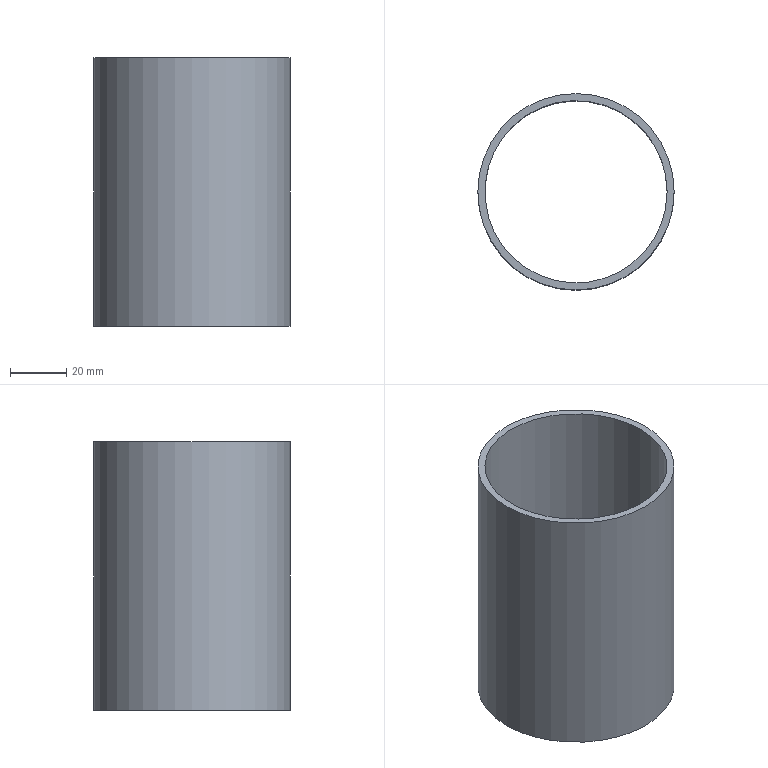Part | NX | features solid 2 | 1 solid | 158 faces | box 69.5 x 69.5 x 95 mm | volume 49985 mm3 | plane 101 | spline 55 | cylinder 2 | commonest cylinder face diameters 64.5 x1 69.5 x1